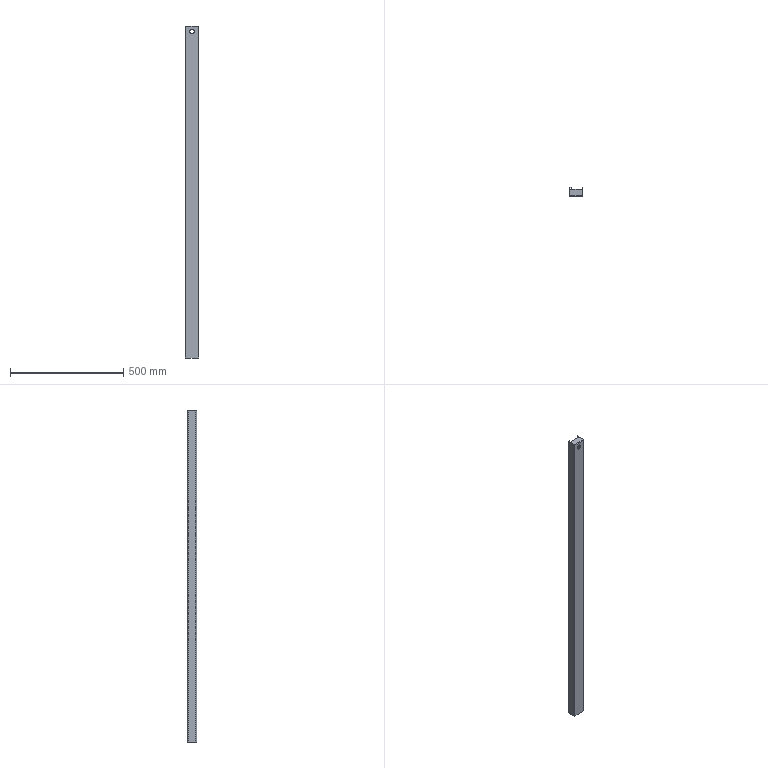Part | STEP file | Sliding Door Upper Rail | 1 solid | 30 faces | box 60 x 40 x 1467 mm | volume 413342 mm3 | plane 20 | cylinder 10 | commonest cylinder face diameters 1 x4 5 x4 20 x2
STEP:
#1=CARTESIAN_POINT('',(-4.447,-19.436,1432.));
#2=VERTEX_POINT('',#1);
#3=CARTESIAN_POINT('',(-4.447,-19.436,1452.));
#4=VERTEX_POINT('',#3);
#5=CARTESIAN_POINT('',(-4.447,-19.436,1442.));
#6=DIRECTION('',(0.,1.,0.));
#7=DIRECTION('',(0.,0.,1.));
#8=AXIS2_PLACEMENT_3D('',#5,#6,#7);
#9=CIRCLE('',#8,10.);
#10=EDGE_CURVE('',#2,#4,#9,.T.);
#11=ORIENTED_EDGE('',*,*,#10,.F.);
#12=CARTESIAN_POINT('',(-4.447,-17.436,1432.));
#13=VERTEX_POINT('',#12);
#14=CARTESIAN_POINT('',(-4.447,-27.436,1432.));
#15=DIRECTION('',(0.,1.,0.));
#16=VECTOR('',#15,1000.);
#17=LINE('',#14,#16);
#18=EDGE_CURVE('',#2,#13,#17,.T.);
#19=ORIENTED_EDGE('',*,*,#18,.T.);
#20=CARTESIAN_POINT('',(-4.447,-17.436,1452.));
#21=VERTEX_POINT('',#20);
#22=CARTESIAN_POINT('',(-4.447,-17.436,1442.));
#23=DIRECTION('',(0.,-1.,0.));
#24=DIRECTION('',(0.,0.,1.));
#25=AXIS2_PLACEMENT_3D('',#22,#23,#24);
#26=CIRCLE('',#25,10.);
#27=EDGE_CURVE('',#21,#13,#26,.T.);
#28=ORIENTED_EDGE('',*,*,#27,.F.);
#29=CARTESIAN_POINT('',(-4.447,-27.436,1452.));
#30=DIRECTION('',(0.,1.,0.));
#31=VECTOR('',#30,1000.);
#32=LINE('',#29,#31);
#33=EDGE_CURVE('',#4,#21,#32,.T.);
#34=ORIENTED_EDGE('',*,*,#33,.F.);
#35=EDGE_LOOP('',(#11,#19,#28,#34));
#36=FACE_OUTER_BOUND('',#35,.T.);
#37=CARTESIAN_POINT('',(-4.447,-27.436,1442.));
#38=DIRECTION('',(0.,1.,0.));
#39=DIRECTION('',(0.,0.,1.));
#40=AXIS2_PLACEMENT_3D('',#37,#38,#39);
#41=CYLINDRICAL_SURFACE('',#40,10.);
#42=ADVANCED_FACE('',(#36),#41,.F.);
#43=CARTESIAN_POINT('',(23.053,-17.436,1464.5));
#44=VERTEX_POINT('',#43);
#45=CARTESIAN_POINT('',(23.053,-17.436,0.));
#46=VERTEX_POINT('',#45);
#47=CARTESIAN_POINT('',(23.053,-17.436,1467.));
#48=DIRECTION('',(0.,0.,-1.));
#49=VECTOR('',#48,1000.);
#50=LINE('',#47,#49);
#51=EDGE_CURVE('',#44,#46,#50,.T.);
#52=ORIENTED_EDGE('',*,*,#51,.T.);
#53=CARTESIAN_POINT('',(-31.947,-17.436,0.));
#54=VERTEX_POINT('',#53);
#55=CARTESIAN_POINT('',(-34.447,-17.436,0.));
#56=DIRECTION('',(-1.,0.,0.));
#57=VECTOR('',#56,1000.);
#58=LINE('',#55,#57);
#59=EDGE_CURVE('',#46,#54,#58,.T.);
#60=ORIENTED_EDGE('',*,*,#59,.T.);
#61=CARTESIAN_POINT('',(-31.947,-17.436,1464.5));
#62=VERTEX_POINT('',#61);
#63=CARTESIAN_POINT('',(-31.947,-17.436,1467.));
#64=DIRECTION('',(0.,0.,1.));
#65=VECTOR('',#64,1000.);
#66=LINE('',#63,#65);
#67=EDGE_CURVE('',#54,#62,#66,.T.);
#68=ORIENTED_EDGE('',*,*,#67,.T.);
#69=CARTESIAN_POINT('',(-34.447,-17.436,1464.5));
#70=DIRECTION('',(1.,0.,0.));
#71=VECTOR('',#70,1000.);
#72=LINE('',#69,#71);
#73=EDGE_CURVE('',#62,#44,#72,.T.);
#74=ORIENTED_EDGE('',*,*,#73,.T.);
#75=EDGE_LOOP('',(#52,#60,#68,#74));
#76=FACE_OUTER_BOUND('',#75,.T.);
#77=ORIENTED_EDGE('',*,*,#27,.T.);
#78=CARTESIAN_POINT('',(-4.447,-17.436,1442.));
#79=DIRECTION('',(0.,-1.,0.));
#80=DIRECTION('',(0.,0.,1.));
#81=AXIS2_PLACEMENT_3D('',#78,#79,#80);
#82=CIRCLE('',#81,10.);
#83=EDGE_CURVE('',#13,#21,#82,.T.);
#84=ORIENTED_EDGE('',*,*,#83,.T.);
#85=EDGE_LOOP('',(#77,#84));
#86=FACE_BOUND('',#85,.T.);
#87=CARTESIAN_POINT('',(-34.447,-17.436,1467.));
#88=DIRECTION('',(0.,1.,0.));
#89=DIRECTION('',(0.,0.,1.));
#90=AXIS2_PLACEMENT_3D('',#87,#88,#89);
#91=PLANE('',#90);
#92=ADVANCED_FACE('',(#76,#86),#91,.T.);
#93=ORIENTED_EDGE('',*,*,#59,.F.);
#94=CARTESIAN_POINT('',(23.553,-16.936,0.));
#95=VERTEX_POINT('',#94);
#96=CARTESIAN_POINT('',(23.053,-16.936,0.));
#97=DIRECTION('',(0.,0.,1.));
#98=DIRECTION('',(-1.,0.,0.));
#99=AXIS2_PLACEMENT_3D('',#96,#97,#98);
#100=CIRCLE('',#99,0.5);
#101=EDGE_CURVE('',#46,#95,#100,.T.);
#102=ORIENTED_EDGE('',*,*,#101,.T.);
#103=CARTESIAN_POINT('',(23.553,20.564,0.));
#104=VERTEX_POINT('',#103);
#105=CARTESIAN_POINT('',(23.553,-19.436,0.));
#106=DIRECTION('',(0.,-1.,0.));
#107=VECTOR('',#106,1000.);
#108=LINE('',#105,#107);
#109=EDGE_CURVE('',#104,#95,#108,.T.);
#110=ORIENTED_EDGE('',*,*,#109,.F.);
#111=CARTESIAN_POINT('',(25.553,20.564,0.));
#112=VERTEX_POINT('',#111);
#113=CARTESIAN_POINT('',(23.053,20.564,0.));
#114=DIRECTION('',(1.,0.,0.));
#115=VECTOR('',#114,1000.);
#116=LINE('',#113,#115);
#117=EDGE_CURVE('',#104,#112,#116,.T.);
#118=ORIENTED_EDGE('',*,*,#117,.T.);
#119=CARTESIAN_POINT('',(25.553,-16.936,0.));
#120=VERTEX_POINT('',#119);
#121=CARTESIAN_POINT('',(25.553,-17.436,0.));
#122=DIRECTION('',(0.,-1.,0.));
#123=VECTOR('',#122,1000.);
#124=LINE('',#121,#123);
#125=EDGE_CURVE('',#112,#120,#124,.T.);
#126=ORIENTED_EDGE('',*,*,#125,.T.);
#127=CARTESIAN_POINT('',(23.053,-19.436,0.));
#128=VERTEX_POINT('',#127);
#129=CARTESIAN_POINT('',(23.053,-16.936,0.));
#130=DIRECTION('',(0.,0.,-1.));
#131=DIRECTION('',(-1.,0.,0.));
#132=AXIS2_PLACEMENT_3D('',#129,#130,#131);
#133=CIRCLE('',#132,2.5);
#134=EDGE_CURVE('',#120,#128,#133,.T.);
#135=ORIENTED_EDGE('',*,*,#134,.T.);
#136=CARTESIAN_POINT('',(-31.947,-19.436,0.));
#137=VERTEX_POINT('',#136);
#138=CARTESIAN_POINT('',(-32.447,-19.436,0.));
#139=DIRECTION('',(-1.,0.,0.));
#140=VECTOR('',#139,1000.);
#141=LINE('',#138,#140);
#142=EDGE_CURVE('',#128,#137,#141,.T.);
#143=ORIENTED_EDGE('',*,*,#142,.T.);
#144=CARTESIAN_POINT('',(-34.447,-16.936,0.));
#145=VERTEX_POINT('',#144);
#146=CARTESIAN_POINT('',(-31.947,-16.936,0.));
#147=DIRECTION('',(0.,0.,-1.));
#148=DIRECTION('',(-1.,0.,0.));
#149=AXIS2_PLACEMENT_3D('',#146,#147,#148);
#150=CIRCLE('',#149,2.5);
#151=EDGE_CURVE('',#137,#145,#150,.T.);
#152=ORIENTED_EDGE('',*,*,#151,.T.);
#153=CARTESIAN_POINT('',(-34.447,18.064,0.));
#154=VERTEX_POINT('',#153);
#155=CARTESIAN_POINT('',(-34.447,18.564,0.));
#156=DIRECTION('',(0.,1.,0.));
#157=VECTOR('',#156,1000.);
#158=LINE('',#155,#157);
#159=EDGE_CURVE('',#145,#154,#158,.T.);
#160=ORIENTED_EDGE('',*,*,#159,.T.);
#161=CARTESIAN_POINT('',(-31.947,20.564,0.));
#162=VERTEX_POINT('',#161);
#163=CARTESIAN_POINT('',(-31.947,18.064,0.));
#164=DIRECTION('',(0.,0.,-1.));
#165=DIRECTION('',(-1.,0.,0.));
#166=AXIS2_PLACEMENT_3D('',#163,#164,#165);
#167=CIRCLE('',#166,2.5);
#168=EDGE_CURVE('',#154,#162,#167,.T.);
#169=ORIENTED_EDGE('',*,*,#168,.T.);
#170=CARTESIAN_POINT('',(-26.447,20.564,0.));
#171=VERTEX_POINT('',#170);
#172=CARTESIAN_POINT('',(23.053,20.564,0.));
#173=DIRECTION('',(-1.,0.,0.));
#174=VECTOR('',#173,1000.);
#175=LINE('',#172,#174);
#176=EDGE_CURVE('',#171,#162,#175,.T.);
#177=ORIENTED_EDGE('',*,*,#176,.F.);
#178=CARTESIAN_POINT('',(-26.447,18.564,0.));
#179=VERTEX_POINT('',#178);
#180=CARTESIAN_POINT('',(-26.447,-16.936,0.));
#181=DIRECTION('',(0.,1.,0.));
#182=VECTOR('',#181,1000.);
#183=LINE('',#180,#182);
#184=EDGE_CURVE('',#179,#171,#183,.T.);
#185=ORIENTED_EDGE('',*,*,#184,.F.);
#186=CARTESIAN_POINT('',(-31.947,18.564,0.));
#187=VERTEX_POINT('',#186);
#188=CARTESIAN_POINT('',(-26.447,18.564,0.));
#189=DIRECTION('',(1.,0.,0.));
#190=VECTOR('',#189,1000.);
#191=LINE('',#188,#190);
#192=EDGE_CURVE('',#187,#179,#191,.T.);
#193=ORIENTED_EDGE('',*,*,#192,.F.);
#194=CARTESIAN_POINT('',(-32.447,18.064,0.));
#195=VERTEX_POINT('',#194);
#196=CARTESIAN_POINT('',(-31.947,18.064,0.));
#197=DIRECTION('',(0.,0.,1.));
#198=DIRECTION('',(-1.,0.,0.));
#199=AXIS2_PLACEMENT_3D('',#196,#197,#198);
#200=CIRCLE('',#199,0.5);
#201=EDGE_CURVE('',#187,#195,#200,.T.);
#202=ORIENTED_EDGE('',*,*,#201,.T.);
#203=CARTESIAN_POINT('',(-32.447,-16.936,0.));
#204=VERTEX_POINT('',#203);
#205=CARTESIAN_POINT('',(-32.447,20.564,0.));
#206=DIRECTION('',(0.,1.,0.));
#207=VECTOR('',#206,1000.);
#208=LINE('',#205,#207);
#209=EDGE_CURVE('',#204,#195,#208,.T.);
#210=ORIENTED_EDGE('',*,*,#209,.F.);
#211=CARTESIAN_POINT('',(-31.947,-16.936,0.));
#212=DIRECTION('',(0.,0.,1.));
#213=DIRECTION('',(-1.,0.,0.));
#214=AXIS2_PLACEMENT_3D('',#211,#212,#213);
#215=CIRCLE('',#214,0.5);
#216=EDGE_CURVE('',#204,#54,#215,.T.);
#217=ORIENTED_EDGE('',*,*,#216,.T.);
#218=EDGE_LOOP('',(#93,#102,#110,#118,#126,#135,#143,#152,#160,#169,#177,#185,#193,#202,#210,#217));
#219=FACE_OUTER_BOUND('',#218,.T.);
#220=CARTESIAN_POINT('',(-32.447,-16.936,0.));
#221=DIRECTION('',(0.,0.,-1.));
#222=DIRECTION('',(-1.,0.,0.));
#223=AXIS2_PLACEMENT_3D('',#220,#221,#222);
#224=PLANE('',#223);
#225=ADVANCED_FACE('',(#219),#224,.T.);
#226=ORIENTED_EDGE('',*,*,#51,.F.);
#227=CARTESIAN_POINT('',(23.053,-17.436,1466.949));
#228=VERTEX_POINT('',#227);
#229=CARTESIAN_POINT('',(23.053,-17.436,1467.));
#230=DIRECTION('',(0.,0.,-1.));
#231=VECTOR('',#230,1000.);
#232=LINE('',#229,#231);
#233=EDGE_CURVE('',#228,#44,#232,.T.);
#234=ORIENTED_EDGE('',*,*,#233,.F.);
#235=CARTESIAN_POINT('',(23.053,-17.436,1467.));
#236=VERTEX_POINT('',#235);
#237=CARTESIAN_POINT('',(23.053,-17.436,1467.));
#238=DIRECTION('',(0.,0.,-1.));
#239=VECTOR('',#238,1000.);
#240=LINE('',#237,#239);
#241=EDGE_CURVE('',#236,#228,#240,.T.);
#242=ORIENTED_EDGE('',*,*,#241,.F.);
#243=CARTESIAN_POINT('',(23.553,-16.936,1467.));
#244=VERTEX_POINT('',#243);
#245=CARTESIAN_POINT('',(23.053,-16.936,1467.));
#246=DIRECTION('',(0.,0.,-1.));
#247=DIRECTION('',(-1.,0.,0.));
#248=AXIS2_PLACEMENT_3D('',#245,#246,#247);
#249=CIRCLE('',#248,0.5);
#250=EDGE_CURVE('',#244,#236,#249,.T.);
#251=ORIENTED_EDGE('',*,*,#250,.F.);
#252=CARTESIAN_POINT('',(23.553,-16.936,1467.));
#253=DIRECTION('',(0.,0.,1.));
#254=VECTOR('',#253,1000.);
#255=LINE('',#252,#254);
#256=EDGE_CURVE('',#95,#244,#255,.T.);
#257=ORIENTED_EDGE('',*,*,#256,.F.);
#258=ORIENTED_EDGE('',*,*,#101,.F.);
#259=EDGE_LOOP('',(#226,#234,#242,#251,#257,#258));
#260=FACE_OUTER_BOUND('',#259,.T.);
#261=CARTESIAN_POINT('',(23.053,-16.936,1467.));
#262=DIRECTION('',(0.,0.,-1.));
#263=DIRECTION('',(-1.,0.,0.));
#264=AXIS2_PLACEMENT_3D('',#261,#262,#263);
#265=CYLINDRICAL_SURFACE('',#264,0.5);
#266=ADVANCED_FACE('',(#260),#265,.F.);
#267=CARTESIAN_POINT('',(-31.947,-16.936,1465.));
#268=VERTEX_POINT('',#267);
#269=CARTESIAN_POINT('',(-31.947,-16.936,1464.5));
#270=DIRECTION('',(1.,0.,0.));
#271=DIRECTION('',(0.,0.,-1.));
#272=AXIS2_PLACEMENT_3D('',#269,#270,#271);
#273=CIRCLE('',#272,0.5);
#274=EDGE_CURVE('',#268,#62,#273,.T.);
#275=ORIENTED_EDGE('',*,*,#274,.F.);
#276=CARTESIAN_POINT('',(23.053,-16.936,1465.));
#277=VERTEX_POINT('',#276);
#278=CARTESIAN_POINT('',(23.053,-16.936,1465.));
#279=DIRECTION('',(-1.,0.,0.));
#280=VECTOR('',#279,1000.);
#281=LINE('',#278,#280);
#282=EDGE_CURVE('',#277,#268,#281,.T.);
#283=ORIENTED_EDGE('',*,*,#282,.F.);
#284=CARTESIAN_POINT('',(23.053,-16.936,1464.5));
#285=DIRECTION('',(-1.,0.,0.));
#286=DIRECTION('',(0.,0.,-1.));
#287=AXIS2_PLACEMENT_3D('',#284,#285,#286);
#288=CIRCLE('',#287,0.5);
#289=EDGE_CURVE('',#44,#277,#288,.T.);
#290=ORIENTED_EDGE('',*,*,#289,.F.);
#291=ORIENTED_EDGE('',*,*,#73,.F.);
#292=EDGE_LOOP('',(#275,#283,#290,#291));
#293=FACE_OUTER_BOUND('',#292,.T.);
#294=CARTESIAN_POINT('',(23.053,-16.936,1464.5));
#295=DIRECTION('',(1.,0.,0.));
#296=DIRECTION('',(0.,0.,-1.));
#297=AXIS2_PLACEMENT_3D('',#294,#295,#296);
#298=CYLINDRICAL_SURFACE('',#297,0.5);
#299=ADVANCED_FACE('',(#293),#298,.F.);
#300=CARTESIAN_POINT('',(-32.447,-16.936,1467.));
#301=VERTEX_POINT('',#300);
#302=CARTESIAN_POINT('',(-32.447,-16.936,1467.));
#303=DIRECTION('',(0.,0.,-1.));
#304=VECTOR('',#303,1000.);
#305=LINE('',#302,#304);
#306=EDGE_CURVE('',#301,#204,#305,.T.);
#307=ORIENTED_EDGE('',*,*,#306,.F.);
#308=CARTESIAN_POINT('',(-31.947,-17.436,1467.));
#309=VERTEX_POINT('',#308);
#310=CARTESIAN_POINT('',(-31.947,-16.936,1467.));
#311=DIRECTION('',(0.,0.,-1.));
#312=DIRECTION('',(-1.,0.,0.));
#313=AXIS2_PLACEMENT_3D('',#310,#311,#312);
#314=CIRCLE('',#313,0.5);
#315=EDGE_CURVE('',#309,#301,#314,.T.);
#316=ORIENTED_EDGE('',*,*,#315,.F.);
#317=CARTESIAN_POINT('',(-31.947,-17.436,1466.949));
#318=VERTEX_POINT('',#317);
#319=CARTESIAN_POINT('',(-31.947,-17.436,1464.5));
#320=DIRECTION('',(0.,0.,1.));
#321=VECTOR('',#320,1000.);
#322=LINE('',#319,#321);
#323=EDGE_CURVE('',#318,#309,#322,.T.);
#324=ORIENTED_EDGE('',*,*,#323,.F.);
#325=CARTESIAN_POINT('',(-31.947,-17.436,1467.));
#326=DIRECTION('',(0.,0.,1.));
#327=VECTOR('',#326,1000.);
#328=LINE('',#325,#327);
#329=EDGE_CURVE('',#62,#318,#328,.T.);
#330=ORIENTED_EDGE('',*,*,#329,.F.);
#331=ORIENTED_EDGE('',*,*,#67,.F.);
#332=ORIENTED_EDGE('',*,*,#216,.F.);
#333=EDGE_LOOP('',(#307,#316,#324,#330,#331,#332));
#334=FACE_OUTER_BOUND('',#333,.T.);
#335=CARTESIAN_POINT('',(-31.947,-16.936,1467.));
#336=DIRECTION('',(0.,0.,-1.));
#337=DIRECTION('',(-1.,0.,0.));
#338=AXIS2_PLACEMENT_3D('',#335,#336,#337);
#339=CYLINDRICAL_SURFACE('',#338,0.5);
#340=ADVANCED_FACE('',(#334),#339,.F.);
#341=ORIENTED_EDGE('',*,*,#18,.F.);
#342=CARTESIAN_POINT('',(-4.447,-19.436,1442.));
#343=DIRECTION('',(0.,1.,0.));
#344=DIRECTION('',(0.,0.,1.));
#345=AXIS2_PLACEMENT_3D('',#342,#343,#344);
#346=CIRCLE('',#345,10.);
#347=EDGE_CURVE('',#4,#2,#346,.T.);
#348=ORIENTED_EDGE('',*,*,#347,.F.);
#349=ORIENTED_EDGE('',*,*,#33,.T.);
#350=ORIENTED_EDGE('',*,*,#83,.F.);
#351=EDGE_LOOP('',(#341,#348,#349,#350));
#352=FACE_OUTER_BOUND('',#351,.T.);
#353=CARTESIAN_POINT('',(-4.447,-27.436,1442.));
#354=DIRECTION('',(0.,1.,0.));
#355=DIRECTION('',(0.,0.,1.));
#356=AXIS2_PLACEMENT_3D('',#353,#354,#355);
#357=CYLINDRICAL_SURFACE('',#356,10.);
#358=ADVANCED_FACE('',(#352),#357,.F.);
#359=CARTESIAN_POINT('',(-31.947,-19.436,1464.5));
#360=VERTEX_POINT('',#359);
#361=CARTESIAN_POINT('',(-31.947,-19.436,1467.));
#362=DIRECTION('',(0.,0.,1.));
#363=VECTOR('',#362,1000.);
#364=LINE('',#361,#363);
#365=EDGE_CURVE('',#137,#360,#364,.T.);
#366=ORIENTED_EDGE('',*,*,#365,.F.);
#367=ORIENTED_EDGE('',*,*,#142,.F.);
#368=CARTESIAN_POINT('',(23.053,-19.436,1464.5));
#369=VERTEX_POINT('',#368);
#370=CARTESIAN_POINT('',(23.053,-19.436,1467.));
#371=DIRECTION('',(0.,0.,-1.));
#372=VECTOR('',#371,1000.);
#373=LINE('',#370,#372);
#374=EDGE_CURVE('',#369,#128,#373,.T.);
#375=ORIENTED_EDGE('',*,*,#374,.F.);
#376=CARTESIAN_POINT('',(-34.447,-19.436,1464.5));
#377=DIRECTION('',(1.,0.,0.));
#378=VECTOR('',#377,1000.);
#379=LINE('',#376,#378);
#380=EDGE_CURVE('',#360,#369,#379,.T.);
#381=ORIENTED_EDGE('',*,*,#380,.F.);
#382=EDGE_LOOP('',(#366,#367,#375,#381));
#383=FACE_OUTER_BOUND('',#382,.T.);
#384=ORIENTED_EDGE('',*,*,#347,.T.);
#385=ORIENTED_EDGE('',*,*,#10,.T.);
#386=EDGE_LOOP('',(#384,#385));
#387=FACE_BOUND('',#386,.T.);
#388=CARTESIAN_POINT('',(-34.447,-19.436,1467.));
#389=DIRECTION('',(0.,1.,0.));
#390=DIRECTION('',(0.,0.,1.));
#391=AXIS2_PLACEMENT_3D('',#388,#389,#390);
#392=PLANE('',#391);
#393=ADVANCED_FACE('',(#383,#387),#392,.F.);
#394=ORIENTED_EDGE('',*,*,#233,.T.);
#395=ORIENTED_EDGE('',*,*,#289,.T.);
#396=CARTESIAN_POINT('',(23.053,10.564,1465.));
#397=VERTEX_POINT('',#396);
#398=CARTESIAN_POINT('',(23.053,0.,1465.));
#399=DIRECTION('',(0.,1.,0.));
#400=VECTOR('',#399,1000.);
#401=LINE('',#398,#400);
#402=EDGE_CURVE('',#277,#397,#401,.T.);
#403=ORIENTED_EDGE('',*,*,#402,.T.);
#404=CARTESIAN_POINT('',(23.053,10.564,1467.));
#405=VERTEX_POINT('',#404);
#406=CARTESIAN_POINT('',(23.053,10.564,1467.));
#407=DIRECTION('',(0.,0.,1.));
#408=VECTOR('',#407,1000.);
#409=LINE('',#406,#408);
#410=EDGE_CURVE('',#397,#405,#409,.T.);
#411=ORIENTED_EDGE('',*,*,#410,.T.);
#412=CARTESIAN_POINT('',(23.053,-16.936,1467.));
#413=VERTEX_POINT('',#412);
#414=CARTESIAN_POINT('',(23.053,-17.436,1467.));
#415=DIRECTION('',(0.,-1.,0.));
#416=VECTOR('',#415,1000.);
#417=LINE('',#414,#416);
#418=EDGE_CURVE('',#405,#413,#417,.T.);
#419=ORIENTED_EDGE('',*,*,#418,.T.);
#420=CARTESIAN_POINT('',(23.053,-16.936,1464.5));
#421=DIRECTION('',(-1.,0.,0.));
#422=DIRECTION('',(0.,0.,-1.));
#423=AXIS2_PLACEMENT_3D('',#420,#421,#422);
#424=CIRCLE('',#423,2.5);
#425=EDGE_CURVE('',#228,#413,#424,.T.);
#426=ORIENTED_EDGE('',*,*,#425,.F.);
#427=EDGE_LOOP('',(#394,#395,#403,#411,#419,#426));
#428=FACE_OUTER_BOUND('',#427,.T.);
#429=CARTESIAN_POINT('',(23.053,-16.936,1464.5));
#430=DIRECTION('',(-1.,0.,0.));
#431=DIRECTION('',(0.,0.,1.));
#432=AXIS2_PLACEMENT_3D('',#429,#430,#431);
#433=PLANE('',#432);
#434=ADVANCED_FACE('',(#428),#433,.F.);
#435=CARTESIAN_POINT('',(23.553,20.564,1467.));
#436=VERTEX_POINT('',#435);
#437=CARTESIAN_POINT('',(23.553,-19.436,1467.));
#438=DIRECTION('',(0.,1.,0.));
#439=VECTOR('',#438,1000.);
#440=LINE('',#437,#439);
#441=EDGE_CURVE('',#244,#436,#440,.T.);
#442=ORIENTED_EDGE('',*,*,#441,.T.);
#443=CARTESIAN_POINT('',(23.553,20.564,1467.));
#444=DIRECTION('',(0.,0.,-1.));
#445=VECTOR('',#444,1000.);
#446=LINE('',#443,#445);
#447=EDGE_CURVE('',#436,#104,#446,.T.);
#448=ORIENTED_EDGE('',*,*,#447,.T.);
#449=ORIENTED_EDGE('',*,*,#109,.T.);
#450=ORIENTED_EDGE('',*,*,#256,.T.);
#451=EDGE_LOOP('',(#442,#448,#449,#450));
#452=FACE_OUTER_BOUND('',#451,.T.);
#453=CARTESIAN_POINT('',(23.553,-19.436,1467.));
#454=DIRECTION('',(-1.,0.,0.));
#455=DIRECTION('',(0.,0.,1.));
#456=AXIS2_PLACEMENT_3D('',#453,#454,#455);
#457=PLANE('',#456);
#458=ADVANCED_FACE('',(#452),#457,.T.);
#459=CARTESIAN_POINT('',(-31.947,10.564,1465.));
#460=VERTEX_POINT('',#459);
#461=CARTESIAN_POINT('',(-31.947,0.,1465.));
#462=DIRECTION('',(0.,-1.,0.));
#463=VECTOR('',#462,1000.);
#464=LINE('',#461,#463);
#465=EDGE_CURVE('',#460,#268,#464,.T.);
#466=ORIENTED_EDGE('',*,*,#465,.F.);
#467=CARTESIAN_POINT('',(0.,10.564,1465.));
#468=DIRECTION('',(-1.,0.,0.));
#469=VECTOR('',#468,1000.);
#470=LINE('',#467,#469);
#471=EDGE_CURVE('',#397,#460,#470,.T.);
#472=ORIENTED_EDGE('',*,*,#471,.F.);
#473=ORIENTED_EDGE('',*,*,#402,.F.);
#474=ORIENTED_EDGE('',*,*,#282,.T.);
#475=EDGE_LOOP('',(#466,#472,#473,#474));
#476=FACE_OUTER_BOUND('',#475,.T.);
#477=CARTESIAN_POINT('',(0.,0.,1465.));
#478=DIRECTION('',(0.,0.,1.));
#479=DIRECTION('',(1.,0.,0.));
#480=AXIS2_PLACEMENT_3D('',#477,#478,#479);
#481=PLANE('',#480);
#482=ADVANCED_FACE('',(#476),#481,.F.);
#483=CARTESIAN_POINT('',(-32.447,18.064,1467.));
#484=VERTEX_POINT('',#483);
#485=CARTESIAN_POINT('',(-32.447,20.564,1467.));
#486=DIRECTION('',(0.,-1.,0.));
#487=VECTOR('',#486,1000.);
#488=LINE('',#485,#487);
#489=EDGE_CURVE('',#484,#301,#488,.T.);
#490=ORIENTED_EDGE('',*,*,#489,.T.);
#491=ORIENTED_EDGE('',*,*,#306,.T.);
#492=ORIENTED_EDGE('',*,*,#209,.T.);
#493=CARTESIAN_POINT('',(-32.447,18.064,1467.));
#494=DIRECTION('',(0.,0.,1.));
#495=VECTOR('',#494,1000.);
#496=LINE('',#493,#495);
#497=EDGE_CURVE('',#195,#484,#496,.T.);
#498=ORIENTED_EDGE('',*,*,#497,.T.);
#499=EDGE_LOOP('',(#490,#491,#492,#498));
#500=FACE_OUTER_BOUND('',#499,.T.);
#501=CARTESIAN_POINT('',(-32.447,20.564,1467.));
#502=DIRECTION('',(1.,0.,0.));
#503=DIRECTION('',(0.,0.,-1.));
#504=AXIS2_PLACEMENT_3D('',#501,#502,#503);
#505=PLANE('',#504);
#506=ADVANCED_FACE('',(#500),#505,.T.);
#507=CARTESIAN_POINT('',(-31.947,-16.936,1467.));
#508=VERTEX_POINT('',#507);
#509=CARTESIAN_POINT('',(-31.947,-16.936,1464.5));
#510=DIRECTION('',(-1.,0.,0.));
#511=DIRECTION('',(0.,0.,-1.));
#512=AXIS2_PLACEMENT_3D('',#509,#510,#511);
#513=CIRCLE('',#512,2.5);
#514=EDGE_CURVE('',#318,#508,#513,.T.);
#515=ORIENTED_EDGE('',*,*,#514,.T.);
#516=CARTESIAN_POINT('',(-31.947,10.564,1467.));
#517=VERTEX_POINT('',#516);
#518=CARTESIAN_POINT('',(-31.947,10.564,1467.));
#519=DIRECTION('',(0.,1.,0.));
#520=VECTOR('',#519,1000.);
#521=LINE('',#518,#520);
#522=EDGE_CURVE('',#508,#517,#521,.T.);
#523=ORIENTED_EDGE('',*,*,#522,.T.);
#524=CARTESIAN_POINT('',(-31.947,10.564,1467.));
#525=DIRECTION('',(0.,0.,-1.));
#526=VECTOR('',#525,1000.);
#527=LINE('',#524,#526);
#528=EDGE_CURVE('',#517,#460,#527,.T.);
#529=ORIENTED_EDGE('',*,*,#528,.T.);
#530=ORIENTED_EDGE('',*,*,#465,.T.);
#531=ORIENTED_EDGE('',*,*,#274,.T.);
#532=ORIENTED_EDGE('',*,*,#329,.T.);
#533=EDGE_LOOP('',(#515,#523,#529,#530,#531,#532));
#534=FACE_OUTER_BOUND('',#533,.T.);
#535=CARTESIAN_POINT('',(-31.947,-16.936,1464.5));
#536=DIRECTION('',(-1.,0.,0.));
#537=DIRECTION('',(0.,0.,1.));
#538=AXIS2_PLACEMENT_3D('',#535,#536,#537);
#539=PLANE('',#538);
#540=ADVANCED_FACE('',(#534),#539,.T.);
#541=CARTESIAN_POINT('',(23.053,-19.436,1467.));
#542=VERTEX_POINT('',#541);
#543=CARTESIAN_POINT('',(23.053,-19.436,1467.));
#544=DIRECTION('',(0.,0.,-1.));
#545=VECTOR('',#544,1000.);
#546=LINE('',#543,#545);
#547=EDGE_CURVE('',#542,#369,#546,.T.);
#548=ORIENTED_EDGE('',*,*,#547,.T.);
#549=ORIENTED_EDGE('',*,*,#374,.T.);
#550=ORIENTED_EDGE('',*,*,#134,.F.);
#551=CARTESIAN_POINT('',(25.553,-16.936,1467.));
#552=VERTEX_POINT('',#551);
#553=CARTESIAN_POINT('',(25.553,-16.936,1467.));
#554=DIRECTION('',(0.,0.,1.));
#555=VECTOR('',#554,1000.);
#556=LINE('',#553,#555);
#557=EDGE_CURVE('',#120,#552,#556,.T.);
#558=ORIENTED_EDGE('',*,*,#557,.T.);
#559=CARTESIAN_POINT('',(23.053,-16.936,1467.));
#560=DIRECTION('',(0.,0.,-1.));
#561=DIRECTION('',(-1.,0.,0.));
#562=AXIS2_PLACEMENT_3D('',#559,#560,#561);
#563=CIRCLE('',#562,2.5);
#564=EDGE_CURVE('',#552,#542,#563,.T.);
#565=ORIENTED_EDGE('',*,*,#564,.T.);
#566=EDGE_LOOP('',(#548,#549,#550,#558,#565));
#567=FACE_OUTER_BOUND('',#566,.T.);
#568=CARTESIAN_POINT('',(23.053,-16.936,1467.));
#569=DIRECTION('',(0.,0.,-1.));
#570=DIRECTION('',(-1.,0.,0.));
#571=AXIS2_PLACEMENT_3D('',#568,#569,#570);
#572=CYLINDRICAL_SURFACE('',#571,2.5);
#573=ADVANCED_FACE('',(#567),#572,.T.);
#574=CARTESIAN_POINT('',(-31.947,-19.436,1467.));
#575=VERTEX_POINT('',#574);
#576=CARTESIAN_POINT('',(-34.447,-16.936,1467.));
#577=VERTEX_POINT('',#576);
#578=CARTESIAN_POINT('',(-31.947,-16.936,1467.));
#579=DIRECTION('',(0.,0.,-1.));
#580=DIRECTION('',(-1.,0.,0.));
#581=AXIS2_PLACEMENT_3D('',#578,#579,#580);
#582=CIRCLE('',#581,2.5);
#583=EDGE_CURVE('',#575,#577,#582,.T.);
#584=ORIENTED_EDGE('',*,*,#583,.T.);
#585=CARTESIAN_POINT('',(-34.447,-16.936,1467.));
#586=DIRECTION('',(0.,0.,-1.));
#587=VECTOR('',#586,1000.);
#588=LINE('',#585,#587);
#589=EDGE_CURVE('',#577,#145,#588,.T.);
#590=ORIENTED_EDGE('',*,*,#589,.T.);
#591=ORIENTED_EDGE('',*,*,#151,.F.);
#592=ORIENTED_EDGE('',*,*,#365,.T.);
#593=CARTESIAN_POINT('',(-31.947,-19.436,1467.));
#594=DIRECTION('',(0.,0.,1.));
#595=VECTOR('',#594,1000.);
#596=LINE('',#593,#595);
#597=EDGE_CURVE('',#360,#575,#596,.T.);
#598=ORIENTED_EDGE('',*,*,#597,.T.);
#599=EDGE_LOOP('',(#584,#590,#591,#592,#598));
#600=FACE_OUTER_BOUND('',#599,.T.);
#601=CARTESIAN_POINT('',(-31.947,-16.936,1467.));
#602=DIRECTION('',(0.,0.,-1.));
#603=DIRECTION('',(-1.,0.,0.));
#604=AXIS2_PLACEMENT_3D('',#601,#602,#603);
#605=CYLINDRICAL_SURFACE('',#604,2.5);
#606=ADVANCED_FACE('',(#600),#605,.T.);
#607=ORIENTED_EDGE('',*,*,#514,.F.);
#608=CARTESIAN_POINT('',(-31.947,-16.936,1464.5));
#609=DIRECTION('',(1.,0.,0.));
#610=DIRECTION('',(0.,0.,-1.));
#611=AXIS2_PLACEMENT_3D('',#608,#609,#610);
#612=CIRCLE('',#611,2.5);
#613=EDGE_CURVE('',#318,#360,#612,.T.);
#614=ORIENTED_EDGE('',*,*,#613,.T.);
#615=ORIENTED_EDGE('',*,*,#380,.T.);
#616=CARTESIAN_POINT('',(23.053,-16.936,1464.5));
#617=DIRECTION('',(-1.,0.,0.));
#618=DIRECTION('',(0.,0.,-1.));
#619=AXIS2_PLACEMENT_3D('',#616,#617,#618);
#620=CIRCLE('',#619,2.5);
#621=EDGE_CURVE('',#369,#228,#620,.T.);
#622=ORIENTED_EDGE('',*,*,#621,.T.);
#623=ORIENTED_EDGE('',*,*,#425,.T.);
#624=CARTESIAN_POINT('',(23.053,-16.936,1467.));
#625=DIRECTION('',(-1.,0.,0.));
#626=VECTOR('',#625,1000.);
#627=LINE('',#624,#626);
#628=EDGE_CURVE('',#413,#508,#627,.T.);
#629=ORIENTED_EDGE('',*,*,#628,.T.);
#630=EDGE_LOOP('',(#607,#614,#615,#622,#623,#629));
#631=FACE_OUTER_BOUND('',#630,.T.);
#632=CARTESIAN_POINT('',(23.053,-16.936,1464.5));
#633=DIRECTION('',(1.,0.,0.));
#634=DIRECTION('',(0.,0.,-1.));
#635=AXIS2_PLACEMENT_3D('',#632,#633,#634);
#636=CYLINDRICAL_SURFACE('',#635,2.5);
#637=ADVANCED_FACE('',(#631),#636,.T.);
#638=CARTESIAN_POINT('',(25.553,20.564,1467.));
#639=VERTEX_POINT('',#638);
#640=CARTESIAN_POINT('',(23.553,20.564,1467.));
#641=DIRECTION('',(1.,0.,0.));
#642=VECTOR('',#641,1000.);
#643=LINE('',#640,#642);
#644=EDGE_CURVE('',#436,#639,#643,.T.);
#645=ORIENTED_EDGE('',*,*,#644,.T.);
#646=CARTESIAN_POINT('',(25.553,20.564,1467.));
#647=DIRECTION('',(0.,0.,-1.));
#648=VECTOR('',#647,1000.);
#649=LINE('',#646,#648);
#650=EDGE_CURVE('',#639,#112,#649,.T.);
#651=ORIENTED_EDGE('',*,*,#650,.T.);
#652=ORIENTED_EDGE('',*,*,#117,.F.);
#653=ORIENTED_EDGE('',*,*,#447,.F.);
#654=EDGE_LOOP('',(#645,#651,#652,#653));
#655=FACE_OUTER_BOUND('',#654,.T.);
#656=CARTESIAN_POINT('',(23.553,20.564,1467.));
#657=DIRECTION('',(0.,1.,0.));
#658=DIRECTION('',(0.,0.,1.));
#659=AXIS2_PLACEMENT_3D('',#656,#657,#658);
#660=PLANE('',#659);
#661=ADVANCED_FACE('',(#655),#660,.T.);
#662=ORIENTED_EDGE('',*,*,#441,.F.);
#663=ORIENTED_EDGE('',*,*,#250,.T.);
#664=CARTESIAN_POINT('',(23.053,-17.436,1467.));
#665=DIRECTION('',(0.,1.,0.));
#666=VECTOR('',#665,1000.);
#667=LINE('',#664,#666);
#668=EDGE_CURVE('',#542,#236,#667,.T.);
#669=ORIENTED_EDGE('',*,*,#668,.F.);
#670=ORIENTED_EDGE('',*,*,#564,.F.);
#671=CARTESIAN_POINT('',(25.553,-16.936,1467.));
#672=DIRECTION('',(0.,1.,0.));
#673=VECTOR('',#672,1000.);
#674=LINE('',#671,#673);
#675=EDGE_CURVE('',#552,#639,#674,.T.);
#676=ORIENTED_EDGE('',*,*,#675,.T.);
#677=ORIENTED_EDGE('',*,*,#644,.F.);
#678=EDGE_LOOP('',(#662,#663,#669,#670,#676,#677));
#679=FACE_OUTER_BOUND('',#678,.T.);
#680=CARTESIAN_POINT('',(23.053,-16.936,1467.));
#681=DIRECTION('',(0.,0.,1.));
#682=DIRECTION('',(1.,0.,0.));
#683=AXIS2_PLACEMENT_3D('',#680,#681,#682);
#684=PLANE('',#683);
#685=ADVANCED_FACE('',(#679),#684,.T.);
#686=CARTESIAN_POINT('',(23.053,10.564,1467.));
#687=DIRECTION('',(1.,0.,0.));
#688=VECTOR('',#687,1000.);
#689=LINE('',#686,#688);
#690=EDGE_CURVE('',#517,#405,#689,.T.);
#691=ORIENTED_EDGE('',*,*,#690,.T.);
#692=ORIENTED_EDGE('',*,*,#410,.F.);
#693=ORIENTED_EDGE('',*,*,#471,.T.);
#694=ORIENTED_EDGE('',*,*,#528,.F.);
#695=EDGE_LOOP('',(#691,#692,#693,#694));
#696=FACE_OUTER_BOUND('',#695,.T.);
#697=CARTESIAN_POINT('',(23.053,10.564,1467.));
#698=DIRECTION('',(0.,1.,0.));
#699=DIRECTION('',(0.,0.,1.));
#700=AXIS2_PLACEMENT_3D('',#697,#698,#699);
#701=PLANE('',#700);
#702=ADVANCED_FACE('',(#696),#701,.T.);
#703=ORIENTED_EDGE('',*,*,#489,.F.);
#704=CARTESIAN_POINT('',(-31.947,18.564,1467.));
#705=VERTEX_POINT('',#704);
#706=CARTESIAN_POINT('',(-31.947,18.064,1467.));
#707=DIRECTION('',(0.,0.,-1.));
#708=DIRECTION('',(-1.,0.,0.));
#709=AXIS2_PLACEMENT_3D('',#706,#707,#708);
#710=CIRCLE('',#709,0.5);
#711=EDGE_CURVE('',#484,#705,#710,.T.);
#712=ORIENTED_EDGE('',*,*,#711,.T.);
#713=CARTESIAN_POINT('',(-26.447,18.564,1467.));
#714=VERTEX_POINT('',#713);
#715=CARTESIAN_POINT('',(-26.447,18.564,1467.));
#716=DIRECTION('',(-1.,0.,0.));
#717=VECTOR('',#716,1000.);
#718=LINE('',#715,#717);
#719=EDGE_CURVE('',#714,#705,#718,.T.);
#720=ORIENTED_EDGE('',*,*,#719,.F.);
#721=CARTESIAN_POINT('',(-26.447,20.564,1467.));
#722=VERTEX_POINT('',#721);
#723=CARTESIAN_POINT('',(-26.447,18.064,1467.));
#724=DIRECTION('',(0.,1.,0.));
#725=VECTOR('',#724,1000.);
#726=LINE('',#723,#725);
#727=EDGE_CURVE('',#714,#722,#726,.T.);
#728=ORIENTED_EDGE('',*,*,#727,.T.);
#729=CARTESIAN_POINT('',(-31.947,20.564,1467.));
#730=VERTEX_POINT('',#729);
#731=CARTESIAN_POINT('',(-32.447,20.564,1467.));
#732=DIRECTION('',(-1.,0.,0.));
#733=VECTOR('',#732,1000.);
#734=LINE('',#731,#733);
#735=EDGE_CURVE('',#722,#730,#734,.T.);
#736=ORIENTED_EDGE('',*,*,#735,.T.);
#737=CARTESIAN_POINT('',(-34.447,18.064,1467.));
#738=VERTEX_POINT('',#737);
#739=CARTESIAN_POINT('',(-31.947,18.064,1467.));
#740=DIRECTION('',(0.,0.,1.));
#741=DIRECTION('',(-1.,0.,0.));
#742=AXIS2_PLACEMENT_3D('',#739,#740,#741);
#743=CIRCLE('',#742,2.5);
#744=EDGE_CURVE('',#730,#738,#743,.T.);
#745=ORIENTED_EDGE('',*,*,#744,.T.);
#746=CARTESIAN_POINT('',(-34.447,-17.436,1467.));
#747=DIRECTION('',(0.,-1.,0.));
#748=VECTOR('',#747,1000.);
#749=LINE('',#746,#748);
#750=EDGE_CURVE('',#738,#577,#749,.T.);
#751=ORIENTED_EDGE('',*,*,#750,.T.);
#752=ORIENTED_EDGE('',*,*,#583,.F.);
#753=CARTESIAN_POINT('',(-31.947,-16.936,1467.));
#754=DIRECTION('',(0.,1.,0.));
#755=VECTOR('',#754,1000.);
#756=LINE('',#753,#755);
#757=EDGE_CURVE('',#575,#309,#756,.T.);
#758=ORIENTED_EDGE('',*,*,#757,.T.);
#759=ORIENTED_EDGE('',*,*,#315,.T.);
#760=EDGE_LOOP('',(#703,#712,#720,#728,#736,#745,#751,#752,#758,#759));
#761=FACE_OUTER_BOUND('',#760,.T.);
#762=CARTESIAN_POINT('',(-31.947,-17.436,1467.));
#763=DIRECTION('',(0.,0.,1.));
#764=DIRECTION('',(1.,0.,0.));
#765=AXIS2_PLACEMENT_3D('',#762,#763,#764);
#766=PLANE('',#765);
#767=ADVANCED_FACE('',(#761),#766,.T.);
#768=CARTESIAN_POINT('',(-31.947,18.564,1467.));
#769=DIRECTION('',(0.,0.,-1.));
#770=VECTOR('',#769,1000.);
#771=LINE('',#768,#770);
#772=EDGE_CURVE('',#705,#187,#771,.T.);
#773=ORIENTED_EDGE('',*,*,#772,.F.);
#774=ORIENTED_EDGE('',*,*,#711,.F.);
#775=ORIENTED_EDGE('',*,*,#497,.F.);
#776=ORIENTED_EDGE('',*,*,#201,.F.);
#777=EDGE_LOOP('',(#773,#774,#775,#776));
#778=FACE_OUTER_BOUND('',#777,.T.);
#779=CARTESIAN_POINT('',(-31.947,18.064,1467.));
#780=DIRECTION('',(0.,0.,-1.));
#781=DIRECTION('',(-1.,0.,0.));
#782=AXIS2_PLACEMENT_3D('',#779,#780,#781);
#783=CYLINDRICAL_SURFACE('',#782,0.5);
#784=ADVANCED_FACE('',(#778),#783,.F.);
#785=ORIENTED_EDGE('',*,*,#547,.F.);
#786=ORIENTED_EDGE('',*,*,#668,.T.);
#787=ORIENTED_EDGE('',*,*,#241,.T.);
#788=ORIENTED_EDGE('',*,*,#621,.F.);
#789=EDGE_LOOP('',(#785,#786,#787,#788));
#790=FACE_OUTER_BOUND('',#789,.T.);
#791=CARTESIAN_POINT('',(23.053,-17.436,1467.));
#792=DIRECTION('',(-1.,0.,0.));
#793=DIRECTION('',(0.,0.,1.));
#794=AXIS2_PLACEMENT_3D('',#791,#792,#793);
#795=PLANE('',#794);
#796=ADVANCED_FACE('',(#790),#795,.T.);
#797=ORIENTED_EDGE('',*,*,#650,.F.);
#798=ORIENTED_EDGE('',*,*,#675,.F.);
#799=ORIENTED_EDGE('',*,*,#557,.F.);
#800=ORIENTED_EDGE('',*,*,#125,.F.);
#801=EDGE_LOOP('',(#797,#798,#799,#800));
#802=FACE_OUTER_BOUND('',#801,.T.);
#803=CARTESIAN_POINT('',(25.553,-19.436,1467.));
#804=DIRECTION('',(-1.,0.,0.));
#805=DIRECTION('',(0.,0.,1.));
#806=AXIS2_PLACEMENT_3D('',#803,#804,#805);
#807=PLANE('',#806);
#808=ADVANCED_FACE('',(#802),#807,.F.);
#809=ORIENTED_EDGE('',*,*,#589,.F.);
#810=ORIENTED_EDGE('',*,*,#750,.F.);
#811=CARTESIAN_POINT('',(-34.447,18.064,1467.));
#812=DIRECTION('',(0.,0.,1.));
#813=VECTOR('',#812,1000.);
#814=LINE('',#811,#813);
#815=EDGE_CURVE('',#154,#738,#814,.T.);
#816=ORIENTED_EDGE('',*,*,#815,.F.);
#817=ORIENTED_EDGE('',*,*,#159,.F.);
#818=EDGE_LOOP('',(#809,#810,#816,#817));
#819=FACE_OUTER_BOUND('',#818,.T.);
#820=CARTESIAN_POINT('',(-34.447,20.564,1467.));
#821=DIRECTION('',(1.,0.,0.));
#822=DIRECTION('',(0.,0.,-1.));
#823=AXIS2_PLACEMENT_3D('',#820,#821,#822);
#824=PLANE('',#823);
#825=ADVANCED_FACE('',(#819),#824,.F.);
#826=ORIENTED_EDGE('',*,*,#323,.T.);
#827=ORIENTED_EDGE('',*,*,#757,.F.);
#828=ORIENTED_EDGE('',*,*,#597,.F.);
#829=ORIENTED_EDGE('',*,*,#613,.F.);
#830=EDGE_LOOP('',(#826,#827,#828,#829));
#831=FACE_OUTER_BOUND('',#830,.T.);
#832=CARTESIAN_POINT('',(-31.947,-17.436,1464.5));
#833=DIRECTION('',(1.,0.,0.));
#834=DIRECTION('',(0.,0.,-1.));
#835=AXIS2_PLACEMENT_3D('',#832,#833,#834);
#836=PLANE('',#835);
#837=ADVANCED_FACE('',(#831),#836,.T.);
#838=ORIENTED_EDGE('',*,*,#418,.F.);
#839=ORIENTED_EDGE('',*,*,#690,.F.);
#840=ORIENTED_EDGE('',*,*,#522,.F.);
#841=ORIENTED_EDGE('',*,*,#628,.F.);
#842=EDGE_LOOP('',(#838,#839,#840,#841));
#843=FACE_OUTER_BOUND('',#842,.T.);
#844=CARTESIAN_POINT('',(0.,0.,1467.));
#845=DIRECTION('',(0.,0.,1.));
#846=DIRECTION('',(1.,0.,0.));
#847=AXIS2_PLACEMENT_3D('',#844,#845,#846);
#848=PLANE('',#847);
#849=ADVANCED_FACE('',(#843),#848,.T.);
#850=ORIENTED_EDGE('',*,*,#719,.T.);
#851=ORIENTED_EDGE('',*,*,#772,.T.);
#852=ORIENTED_EDGE('',*,*,#192,.T.);
#853=CARTESIAN_POINT('',(-26.447,18.564,1467.));
#854=DIRECTION('',(0.,0.,1.));
#855=VECTOR('',#854,1000.);
#856=LINE('',#853,#855);
#857=EDGE_CURVE('',#179,#714,#856,.T.);
#858=ORIENTED_EDGE('',*,*,#857,.T.);
#859=EDGE_LOOP('',(#850,#851,#852,#858));
#860=FACE_OUTER_BOUND('',#859,.T.);
#861=CARTESIAN_POINT('',(-26.447,18.564,1467.));
#862=DIRECTION('',(0.,-1.,0.));
#863=DIRECTION('',(0.,0.,-1.));
#864=AXIS2_PLACEMENT_3D('',#861,#862,#863);
#865=PLANE('',#864);
#866=ADVANCED_FACE('',(#860),#865,.T.);
#867=ORIENTED_EDGE('',*,*,#744,.F.);
#868=CARTESIAN_POINT('',(-31.947,20.564,1467.));
#869=DIRECTION('',(0.,0.,-1.));
#870=VECTOR('',#869,1000.);
#871=LINE('',#868,#870);
#872=EDGE_CURVE('',#730,#162,#871,.T.);
#873=ORIENTED_EDGE('',*,*,#872,.T.);
#874=ORIENTED_EDGE('',*,*,#168,.F.);
#875=ORIENTED_EDGE('',*,*,#815,.T.);
#876=EDGE_LOOP('',(#867,#873,#874,#875));
#877=FACE_OUTER_BOUND('',#876,.T.);
#878=CARTESIAN_POINT('',(-31.947,18.064,1467.));
#879=DIRECTION('',(0.,0.,-1.));
#880=DIRECTION('',(-1.,0.,0.));
#881=AXIS2_PLACEMENT_3D('',#878,#879,#880);
#882=CYLINDRICAL_SURFACE('',#881,2.5);
#883=ADVANCED_FACE('',(#877),#882,.T.);
#884=ORIENTED_EDGE('',*,*,#727,.F.);
#885=ORIENTED_EDGE('',*,*,#857,.F.);
#886=ORIENTED_EDGE('',*,*,#184,.T.);
#887=CARTESIAN_POINT('',(-26.447,20.564,1467.));
#888=DIRECTION('',(0.,0.,1.));
#889=VECTOR('',#888,1000.);
#890=LINE('',#887,#889);
#891=EDGE_CURVE('',#171,#722,#890,.T.);
#892=ORIENTED_EDGE('',*,*,#891,.T.);
#893=EDGE_LOOP('',(#884,#885,#886,#892));
#894=FACE_OUTER_BOUND('',#893,.T.);
#895=CARTESIAN_POINT('',(-26.447,20.564,1467.));
#896=DIRECTION('',(1.,0.,0.));
#897=DIRECTION('',(0.,0.,-1.));
#898=AXIS2_PLACEMENT_3D('',#895,#896,#897);
#899=PLANE('',#898);
#900=ADVANCED_FACE('',(#894),#899,.T.);
#901=ORIENTED_EDGE('',*,*,#872,.F.);
#902=ORIENTED_EDGE('',*,*,#735,.F.);
#903=ORIENTED_EDGE('',*,*,#891,.F.);
#904=ORIENTED_EDGE('',*,*,#176,.T.);
#905=EDGE_LOOP('',(#901,#902,#903,#904));
#906=FACE_OUTER_BOUND('',#905,.T.);
#907=CARTESIAN_POINT('',(-26.447,20.564,1467.));
#908=DIRECTION('',(0.,-1.,0.));
#909=DIRECTION('',(0.,0.,-1.));
#910=AXIS2_PLACEMENT_3D('',#907,#908,#909);
#911=PLANE('',#910);
#912=ADVANCED_FACE('',(#906),#911,.F.);
#913=CLOSED_SHELL('',(#42,#92,#225,#266,#299,#340,#358,#393,#434,#458,#482,#506,#540,#573,#606,#637,#661,#685,#702,#767,#784,#796,#808,#825,#837,#849,#866,#883,#900,#912));
#914=MANIFOLD_SOLID_BREP('',#913);
#915=CARTESIAN_POINT('',(0.,0.,0.));
#916=DIRECTION('',(0.,0.,1.));
#917=DIRECTION('',(1.,0.,0.));
#918=AXIS2_PLACEMENT_3D('',#915,#916,#917);
#919=(LENGTH_UNIT()NAMED_UNIT(*)SI_UNIT(.MILLI.,.METRE.));
#920=UNCERTAINTY_MEASURE_WITH_UNIT(LENGTH_MEASURE(0.00001),#919,'','');
#921=(NAMED_UNIT(*)PLANE_ANGLE_UNIT()SI_UNIT($,.RADIAN.));
#922=(NAMED_UNIT(*)SI_UNIT($,.STERADIAN.)SOLID_ANGLE_UNIT());
#923=(GEOMETRIC_REPRESENTATION_CONTEXT(3)GLOBAL_UNCERTAINTY_ASSIGNED_CONTEXT((#920))GLOBAL_UNIT_ASSIGNED_CONTEXT((#919,#921,#922))REPRESENTATION_CONTEXT('',''));
#924=ADVANCED_BREP_SHAPE_REPRESENTATION('',(#914,#918),#923);